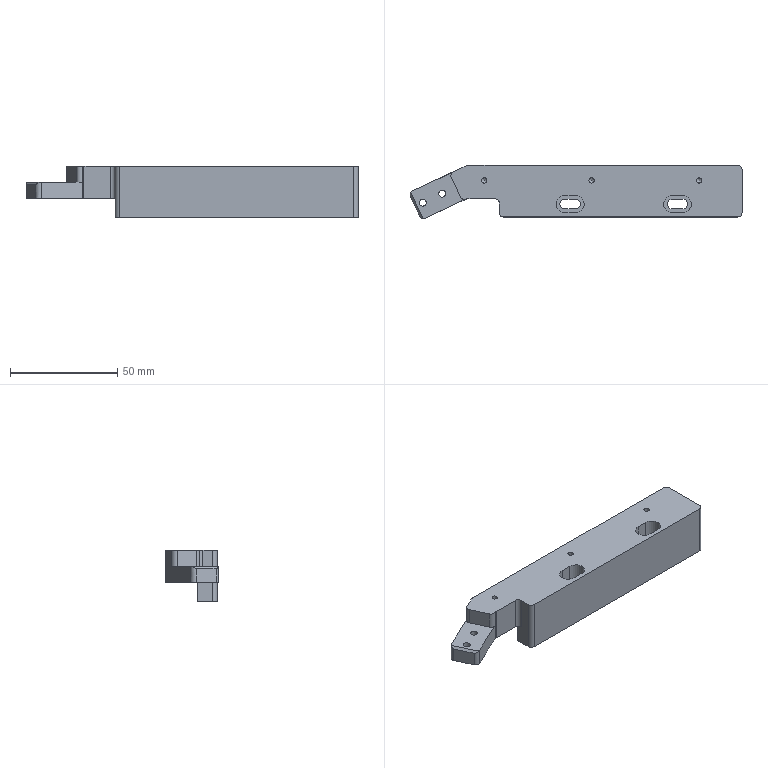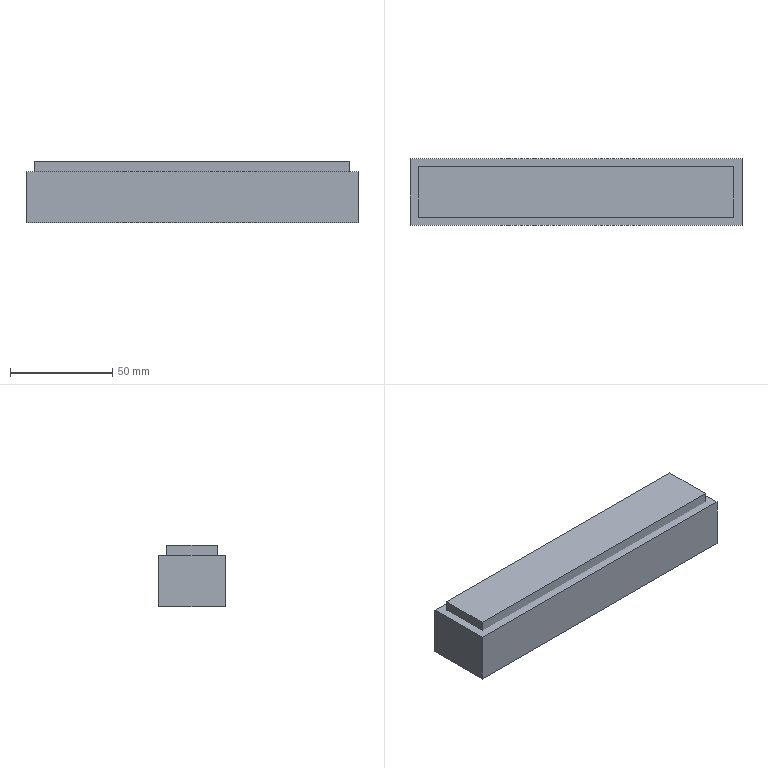CAM job | NX | 3+2 milling, drilling | part box 154.531 x 24.709 x 24 mm | stock box 162.531 x 32.709 x 30 mm
Tools:
number,name,description,diameter,corner_radius,flute_length,length,flutes
1,D50,Milling Tool-5 Parameters,50.0,0.0,50.0,75.0,2
2,D10,Milling Tool-5 Parameters,10.0,0.0,50.0,75.0,2
9,D6A45,Milling Tool-5 Parameters,6.0,0.0,3.0,3.0,2
16,4.2ZT,Drilling Tool,3.2,0.0,35.0,50.0,2
10,2.5ZT,Drilling Tool,2.4,0.0,35.0,50.0,2
4,D6,Milling Tool-5 Parameters,6.0,0.0,50.0,75.0,2
6,D4,Milling Tool-5 Parameters,4.0,0.0,50.0,75.0,2
11,M3XYD,Thread Mill,2.35,0.0,0.5,50.0,2
17,M4XYD,Thread Mill,3.15,0.0,0.7,50.0,2
20,R0.75,Milling Tool-5 Parameters,1.5,0.75,50.0,75.0,2
Operations:
program,operation,operation_type,tool,method,geometry_group,spindle_rpm,surface_speed,feed_per_tooth,feed_cut,feed_plunge,cut_length_mm,path_length_mm,cut_time_min,machine_time_min
1-160-30-30毛胚,FLOOR_WALL,VolumeBased25DMillingOperation,D50,METHOD,A,6500.0,0.0,0.0,1250.0,100.0,224.531,278.531,0.1796,0.185
1-160-30-30毛胚,ADAPTIVE_MILLING,CavityMilling,D10,METHOD,A,7000.0,219.0,0.1429,2000.0,1000.0,7617.049,8518.791,3.817,3.908
1-160-30-30毛胚,ZLEVEL_PROFILE_COPY_COPY_1_COPY,ZLevelMilling,D10,METHOD,A,6500.0,326.0,0.0769,1000.0,1000.0,780.036,885.694,0.78,0.7906
1-160-30-30毛胚,FLOOR_WALL_1_COPY_COPY_1_COPY,VolumeBased25DMillingOperation,D10,METHOD,A,7000.0,219.0,0.0714,1000.0,1000.0,152.745,328.738,0.1527,0.1703
1-160-30-30毛胚,ZLEVEL_PROFILE_COPY_COPY_1_COPY_COPY_1,ZLevelMilling,D6,METHOD,A,7000.0,87.0,0.1,1400.0,1000.0,1201.594,1383.678,0.8779,0.8961
1-160-30-30毛胚,ZLEVEL_PROFILE_COPY_COPY_1_COPY_COPY_1_COPY,ZLevelMilling,D4,METHOD,A,7000.0,87.0,0.0857,1200.0,1000.0,1382.52,1613.868,1.163,1.186
1-160-30-30毛胚,CAVITY_MILL_COPY,CavityMilling,D4,METHOD,A,7000.0,87.0,0.0857,1200.0,1000.0,456.751,834.783,0.3986,0.4364
1-160-30-30毛胚,DRILLING,Operation,D6A45,METHOD,A,4000.0,75.0,0.0312,250.0,0.0,20.0,251.083,0.08,0.1031
1-160-30-30毛胚,DRILLING_COPY_1,Operation,4.2ZT,METHOD,A,2000.0,20.0,0.05,200.0,0.0,25.923,140.286,0.1296,0.1411
1-160-30-30毛胚,THREAD_MILLING_COPY,ThreadMilling,M4XYD,METHOD,A,5000.0,36.0,0.1,1000.0,100.0,1145.294,3287.294,1.145,1.359
1-160-30-30毛胚,DRILLING_COPY_1_COPY,Operation,2.5ZT,METHOD,A,2000.0,20.0,0.05,120.0,0.0,35.13,236.439,0.2927,0.3129
1-160-30-30毛胚,THREAD_MILLING,ThreadMilling,M3XYD,METHOD,A,5000.0,36.0,0.1,1000.0,100.0,347.843,1626.843,0.3478,0.4757
1-160-30-30毛胚,ZLEVEL_PROFILE_COPY_1_COPY_COPY_COPY_COPY,ZLevelMilling,D6A45,METHOD,A,7000.0,131.0,0.0714,1000.0,1000.0,394.486,1124.408,0.3945,0.4675
1-160-30-30毛胚,ZLEVEL_PROFILE_COPY_1_COPY_COPY_COPY_COPY_COPY,ZLevelMilling,D6A45,METHOD,A,7000.0,131.0,0.0714,1000.0,1000.0,62.805,314.826,0.0628,0.088
1-160-30-30毛胚,刀补17,ThreadMilling,M4XYD,METHOD,A,5000.0,36.0,0.1,1000.0,100.0,154.595,328.595,0.1546,0.172
1-160-30-30毛胚,刀补11,ThreadMilling,M3XYD,METHOD,A,5000.0,36.0,0.1,1000.0,100.0,85.013,381.513,0.085,0.1147
2-160-30-30毛胚,FLOOR_WALL_COPY,VolumeBased25DMillingOperation,D50,METHOD,B,6500.0,0.0,0.0,1250.0,100.0,1299.188,2645.847,1.039,1.174
2-160-30-30毛胚,FLOOR_WALL_1,VolumeBased25DMillingOperation,D10,METHOD,B,7000.0,219.0,0.1786,2500.0,1000.0,3661.664,3929.131,1.476,1.502
2-160-30-30毛胚,FLOOR_WALL_1_COPY_COPY_1,VolumeBased25DMillingOperation,D10,METHOD,B,7000.0,219.0,0.0714,1000.0,1000.0,1012.155,1327.772,1.012,1.044
2-160-30-30毛胚,ZLEVEL_PROFILE_COPY_1_COPY_COPY_COPY_COPY_COPY_1,ZLevelMilling,D6A45,METHOD,B,7000.0,131.0,0.0714,1000.0,1000.0,294.765,609.377,0.2948,0.3262
2-160-30-30毛胚,ZLEVEL_PROFILE_COPY_1_COPY_COPY_COPY_COPY_COPY_1_COPY,ZLevelMilling,D6A45,METHOD,B,7000.0,131.0,0.0714,1000.0,1000.0,236.593,626.718,0.2366,0.2756
3-160-30-30毛胚,PLANAR_TEXT,Engraving,R0.75,METHOD,C,7000.0,0.0,0.0,1000.0,500.0,531.071,4575.135,0.607,1.011